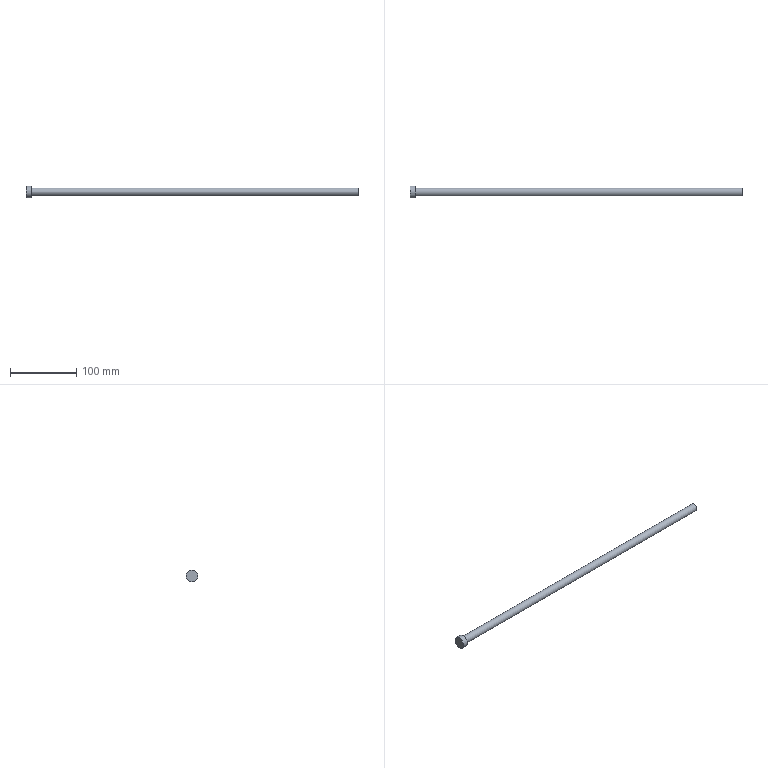Part | STEP file | solid 143 | 1 solid | 5 faces | box 501 x 18 x 18 mm | volume 57793 mm3 | plane 3 | cylinder 2 | commonest cylinder face diameters 12 x1 18 x1